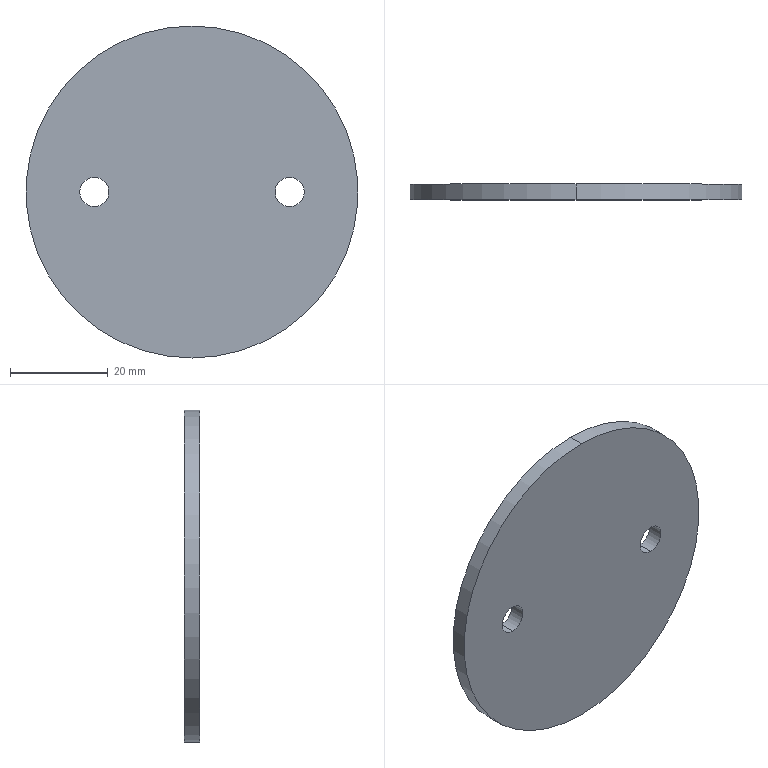Part | SolidWorks | features FlatPattern 1, SMBaseFlange 1, SheetMetal 1 | 1 solid | 8 faces | box 68 x 3.2 x 68 mm | volume 11440 mm3 | cylinder 6 | plane 2 | commonest cylinder face diameters 6 x4 68 x2
STEP:
#1=CARTESIAN_POINT('',(20.,-3.2,-3.));
#2=VERTEX_POINT('',#1);
#3=CARTESIAN_POINT('',(20.,-3.2,3.));
#4=VERTEX_POINT('',#3);
#5=CARTESIAN_POINT('',(20.,-3.2,0.));
#6=DIRECTION('',(0.,1.,0.));
#7=DIRECTION('',(0.,0.,1.));
#8=AXIS2_PLACEMENT_3D('',#5,#6,#7);
#9=CIRCLE('',#8,3.);
#10=EDGE_CURVE('',#2,#4,#9,.T.);
#11=ORIENTED_EDGE('',*,*,#10,.F.);
#12=CARTESIAN_POINT('',(20.,0.,-3.));
#13=VERTEX_POINT('',#12);
#14=CARTESIAN_POINT('',(20.,-3.2,-3.));
#15=DIRECTION('',(0.,1.,0.));
#16=VECTOR('',#15,1000.);
#17=LINE('',#14,#16);
#18=EDGE_CURVE('',#2,#13,#17,.T.);
#19=ORIENTED_EDGE('',*,*,#18,.T.);
#20=CARTESIAN_POINT('',(20.,0.,3.));
#21=VERTEX_POINT('',#20);
#22=CARTESIAN_POINT('',(20.,0.,0.));
#23=DIRECTION('',(0.,1.,0.));
#24=DIRECTION('',(0.,0.,1.));
#25=AXIS2_PLACEMENT_3D('',#22,#23,#24);
#26=CIRCLE('',#25,3.);
#27=EDGE_CURVE('',#13,#21,#26,.T.);
#28=ORIENTED_EDGE('',*,*,#27,.T.);
#29=CARTESIAN_POINT('',(20.,-3.2,3.));
#30=DIRECTION('',(0.,1.,0.));
#31=VECTOR('',#30,1000.);
#32=LINE('',#29,#31);
#33=EDGE_CURVE('',#4,#21,#32,.T.);
#34=ORIENTED_EDGE('',*,*,#33,.F.);
#35=EDGE_LOOP('',(#11,#19,#28,#34));
#36=FACE_OUTER_BOUND('',#35,.T.);
#37=CARTESIAN_POINT('',(20.,-3.2,0.));
#38=DIRECTION('',(0.,1.,0.));
#39=DIRECTION('',(0.,0.,1.));
#40=AXIS2_PLACEMENT_3D('',#37,#38,#39);
#41=CYLINDRICAL_SURFACE('',#40,3.);
#42=ADVANCED_FACE('',(#36),#41,.F.);
#43=CARTESIAN_POINT('',(-20.,-3.2,-3.));
#44=VERTEX_POINT('',#43);
#45=CARTESIAN_POINT('',(-20.,-3.2,3.));
#46=VERTEX_POINT('',#45);
#47=CARTESIAN_POINT('',(-20.,-3.2,0.));
#48=DIRECTION('',(0.,1.,0.));
#49=DIRECTION('',(0.,0.,1.));
#50=AXIS2_PLACEMENT_3D('',#47,#48,#49);
#51=CIRCLE('',#50,3.);
#52=EDGE_CURVE('',#44,#46,#51,.T.);
#53=ORIENTED_EDGE('',*,*,#52,.F.);
#54=CARTESIAN_POINT('',(-20.,0.,-3.));
#55=VERTEX_POINT('',#54);
#56=CARTESIAN_POINT('',(-20.,-3.2,-3.));
#57=DIRECTION('',(0.,1.,0.));
#58=VECTOR('',#57,1000.);
#59=LINE('',#56,#58);
#60=EDGE_CURVE('',#44,#55,#59,.T.);
#61=ORIENTED_EDGE('',*,*,#60,.T.);
#62=CARTESIAN_POINT('',(-20.,0.,3.));
#63=VERTEX_POINT('',#62);
#64=CARTESIAN_POINT('',(-20.,0.,0.));
#65=DIRECTION('',(0.,1.,0.));
#66=DIRECTION('',(0.,0.,1.));
#67=AXIS2_PLACEMENT_3D('',#64,#65,#66);
#68=CIRCLE('',#67,3.);
#69=EDGE_CURVE('',#55,#63,#68,.T.);
#70=ORIENTED_EDGE('',*,*,#69,.T.);
#71=CARTESIAN_POINT('',(-20.,-3.2,3.));
#72=DIRECTION('',(0.,1.,0.));
#73=VECTOR('',#72,1000.);
#74=LINE('',#71,#73);
#75=EDGE_CURVE('',#46,#63,#74,.T.);
#76=ORIENTED_EDGE('',*,*,#75,.F.);
#77=EDGE_LOOP('',(#53,#61,#70,#76));
#78=FACE_OUTER_BOUND('',#77,.T.);
#79=CARTESIAN_POINT('',(-20.,-3.2,0.));
#80=DIRECTION('',(0.,1.,0.));
#81=DIRECTION('',(0.,0.,1.));
#82=AXIS2_PLACEMENT_3D('',#79,#80,#81);
#83=CYLINDRICAL_SURFACE('',#82,3.);
#84=ADVANCED_FACE('',(#78),#83,.F.);
#85=CARTESIAN_POINT('',(0.,-3.2,34.));
#86=VERTEX_POINT('',#85);
#87=CARTESIAN_POINT('',(0.,-3.2,-34.));
#88=VERTEX_POINT('',#87);
#89=CARTESIAN_POINT('',(0.,-3.2,0.));
#90=DIRECTION('',(0.,1.,0.));
#91=DIRECTION('',(0.,0.,1.));
#92=AXIS2_PLACEMENT_3D('',#89,#90,#91);
#93=CIRCLE('',#92,34.);
#94=EDGE_CURVE('',#86,#88,#93,.T.);
#95=ORIENTED_EDGE('',*,*,#94,.T.);
#96=CARTESIAN_POINT('',(0.,0.,-34.));
#97=VERTEX_POINT('',#96);
#98=CARTESIAN_POINT('',(0.,-3.2,-34.));
#99=DIRECTION('',(0.,1.,0.));
#100=VECTOR('',#99,1000.);
#101=LINE('',#98,#100);
#102=EDGE_CURVE('',#88,#97,#101,.T.);
#103=ORIENTED_EDGE('',*,*,#102,.T.);
#104=CARTESIAN_POINT('',(0.,0.,34.));
#105=VERTEX_POINT('',#104);
#106=CARTESIAN_POINT('',(0.,0.,0.));
#107=DIRECTION('',(0.,1.,0.));
#108=DIRECTION('',(0.,0.,1.));
#109=AXIS2_PLACEMENT_3D('',#106,#107,#108);
#110=CIRCLE('',#109,34.);
#111=EDGE_CURVE('',#105,#97,#110,.T.);
#112=ORIENTED_EDGE('',*,*,#111,.F.);
#113=CARTESIAN_POINT('',(0.,-3.2,34.));
#114=DIRECTION('',(0.,1.,0.));
#115=VECTOR('',#114,1000.);
#116=LINE('',#113,#115);
#117=EDGE_CURVE('',#86,#105,#116,.T.);
#118=ORIENTED_EDGE('',*,*,#117,.F.);
#119=EDGE_LOOP('',(#95,#103,#112,#118));
#120=FACE_OUTER_BOUND('',#119,.T.);
#121=CARTESIAN_POINT('',(0.,-3.2,0.));
#122=DIRECTION('',(0.,1.,0.));
#123=DIRECTION('',(0.,0.,1.));
#124=AXIS2_PLACEMENT_3D('',#121,#122,#123);
#125=CYLINDRICAL_SURFACE('',#124,34.);
#126=ADVANCED_FACE('',(#120),#125,.T.);
#127=ORIENTED_EDGE('',*,*,#102,.F.);
#128=CARTESIAN_POINT('',(0.,-3.2,0.));
#129=DIRECTION('',(0.,1.,0.));
#130=DIRECTION('',(0.,0.,1.));
#131=AXIS2_PLACEMENT_3D('',#128,#129,#130);
#132=CIRCLE('',#131,34.);
#133=EDGE_CURVE('',#88,#86,#132,.T.);
#134=ORIENTED_EDGE('',*,*,#133,.T.);
#135=ORIENTED_EDGE('',*,*,#117,.T.);
#136=CARTESIAN_POINT('',(0.,0.,0.));
#137=DIRECTION('',(0.,1.,0.));
#138=DIRECTION('',(0.,0.,1.));
#139=AXIS2_PLACEMENT_3D('',#136,#137,#138);
#140=CIRCLE('',#139,34.);
#141=EDGE_CURVE('',#97,#105,#140,.T.);
#142=ORIENTED_EDGE('',*,*,#141,.F.);
#143=EDGE_LOOP('',(#127,#134,#135,#142));
#144=FACE_OUTER_BOUND('',#143,.T.);
#145=CARTESIAN_POINT('',(0.,-3.2,0.));
#146=DIRECTION('',(0.,1.,0.));
#147=DIRECTION('',(0.,0.,1.));
#148=AXIS2_PLACEMENT_3D('',#145,#146,#147);
#149=CYLINDRICAL_SURFACE('',#148,34.);
#150=ADVANCED_FACE('',(#144),#149,.T.);
#151=CARTESIAN_POINT('',(20.,-3.2,0.));
#152=DIRECTION('',(0.,1.,0.));
#153=DIRECTION('',(0.,0.,1.));
#154=AXIS2_PLACEMENT_3D('',#151,#152,#153);
#155=CIRCLE('',#154,3.);
#156=EDGE_CURVE('',#4,#2,#155,.T.);
#157=ORIENTED_EDGE('',*,*,#156,.T.);
#158=ORIENTED_EDGE('',*,*,#10,.T.);
#159=EDGE_LOOP('',(#157,#158));
#160=FACE_BOUND('',#159,.T.);
#161=CARTESIAN_POINT('',(-20.,-3.2,0.));
#162=DIRECTION('',(0.,1.,0.));
#163=DIRECTION('',(0.,0.,1.));
#164=AXIS2_PLACEMENT_3D('',#161,#162,#163);
#165=CIRCLE('',#164,3.);
#166=EDGE_CURVE('',#46,#44,#165,.T.);
#167=ORIENTED_EDGE('',*,*,#166,.T.);
#168=ORIENTED_EDGE('',*,*,#52,.T.);
#169=EDGE_LOOP('',(#167,#168));
#170=FACE_BOUND('',#169,.T.);
#171=ORIENTED_EDGE('',*,*,#94,.F.);
#172=ORIENTED_EDGE('',*,*,#133,.F.);
#173=EDGE_LOOP('',(#171,#172));
#174=FACE_OUTER_BOUND('',#173,.T.);
#175=CARTESIAN_POINT('',(0.,-3.2,0.));
#176=DIRECTION('',(0.,1.,0.));
#177=DIRECTION('',(0.,0.,1.));
#178=AXIS2_PLACEMENT_3D('',#175,#176,#177);
#179=PLANE('',#178);
#180=ADVANCED_FACE('',(#160,#170,#174),#179,.F.);
#181=CARTESIAN_POINT('',(20.,0.,0.));
#182=DIRECTION('',(0.,1.,0.));
#183=DIRECTION('',(0.,0.,1.));
#184=AXIS2_PLACEMENT_3D('',#181,#182,#183);
#185=CIRCLE('',#184,3.);
#186=EDGE_CURVE('',#21,#13,#185,.T.);
#187=ORIENTED_EDGE('',*,*,#186,.F.);
#188=ORIENTED_EDGE('',*,*,#27,.F.);
#189=EDGE_LOOP('',(#187,#188));
#190=FACE_BOUND('',#189,.T.);
#191=CARTESIAN_POINT('',(-20.,0.,0.));
#192=DIRECTION('',(0.,1.,0.));
#193=DIRECTION('',(0.,0.,1.));
#194=AXIS2_PLACEMENT_3D('',#191,#192,#193);
#195=CIRCLE('',#194,3.);
#196=EDGE_CURVE('',#63,#55,#195,.T.);
#197=ORIENTED_EDGE('',*,*,#196,.F.);
#198=ORIENTED_EDGE('',*,*,#69,.F.);
#199=EDGE_LOOP('',(#197,#198));
#200=FACE_BOUND('',#199,.T.);
#201=ORIENTED_EDGE('',*,*,#111,.T.);
#202=ORIENTED_EDGE('',*,*,#141,.T.);
#203=EDGE_LOOP('',(#201,#202));
#204=FACE_OUTER_BOUND('',#203,.T.);
#205=CARTESIAN_POINT('',(0.,0.,0.));
#206=DIRECTION('',(0.,1.,0.));
#207=DIRECTION('',(0.,0.,1.));
#208=AXIS2_PLACEMENT_3D('',#205,#206,#207);
#209=PLANE('',#208);
#210=ADVANCED_FACE('',(#190,#200,#204),#209,.T.);
#211=ORIENTED_EDGE('',*,*,#60,.F.);
#212=ORIENTED_EDGE('',*,*,#166,.F.);
#213=ORIENTED_EDGE('',*,*,#75,.T.);
#214=ORIENTED_EDGE('',*,*,#196,.T.);
#215=EDGE_LOOP('',(#211,#212,#213,#214));
#216=FACE_OUTER_BOUND('',#215,.T.);
#217=CARTESIAN_POINT('',(-20.,-3.2,0.));
#218=DIRECTION('',(0.,1.,0.));
#219=DIRECTION('',(0.,0.,1.));
#220=AXIS2_PLACEMENT_3D('',#217,#218,#219);
#221=CYLINDRICAL_SURFACE('',#220,3.);
#222=ADVANCED_FACE('',(#216),#221,.F.);
#223=ORIENTED_EDGE('',*,*,#18,.F.);
#224=ORIENTED_EDGE('',*,*,#156,.F.);
#225=ORIENTED_EDGE('',*,*,#33,.T.);
#226=ORIENTED_EDGE('',*,*,#186,.T.);
#227=EDGE_LOOP('',(#223,#224,#225,#226));
#228=FACE_OUTER_BOUND('',#227,.T.);
#229=CARTESIAN_POINT('',(20.,-3.2,0.));
#230=DIRECTION('',(0.,1.,0.));
#231=DIRECTION('',(0.,0.,1.));
#232=AXIS2_PLACEMENT_3D('',#229,#230,#231);
#233=CYLINDRICAL_SURFACE('',#232,3.);
#234=ADVANCED_FACE('',(#228),#233,.F.);
#235=CLOSED_SHELL('',(#42,#84,#126,#150,#180,#210,#222,#234));
#236=MANIFOLD_SOLID_BREP('',#235);
#237=CARTESIAN_POINT('',(0.,0.,0.));
#238=DIRECTION('',(0.,0.,1.));
#239=DIRECTION('',(1.,0.,0.));
#240=AXIS2_PLACEMENT_3D('',#237,#238,#239);
#241=(LENGTH_UNIT()NAMED_UNIT(*)SI_UNIT(.MILLI.,.METRE.));
#242=UNCERTAINTY_MEASURE_WITH_UNIT(LENGTH_MEASURE(0.00001),#241,'','');
#243=(NAMED_UNIT(*)PLANE_ANGLE_UNIT()SI_UNIT($,.RADIAN.));
#244=(NAMED_UNIT(*)SI_UNIT($,.STERADIAN.)SOLID_ANGLE_UNIT());
#245=(GEOMETRIC_REPRESENTATION_CONTEXT(3)GLOBAL_UNCERTAINTY_ASSIGNED_CONTEXT((#242))GLOBAL_UNIT_ASSIGNED_CONTEXT((#241,#243,#244))REPRESENTATION_CONTEXT('',''));
#246=ADVANCED_BREP_SHAPE_REPRESENTATION('',(#236,#240),#245);